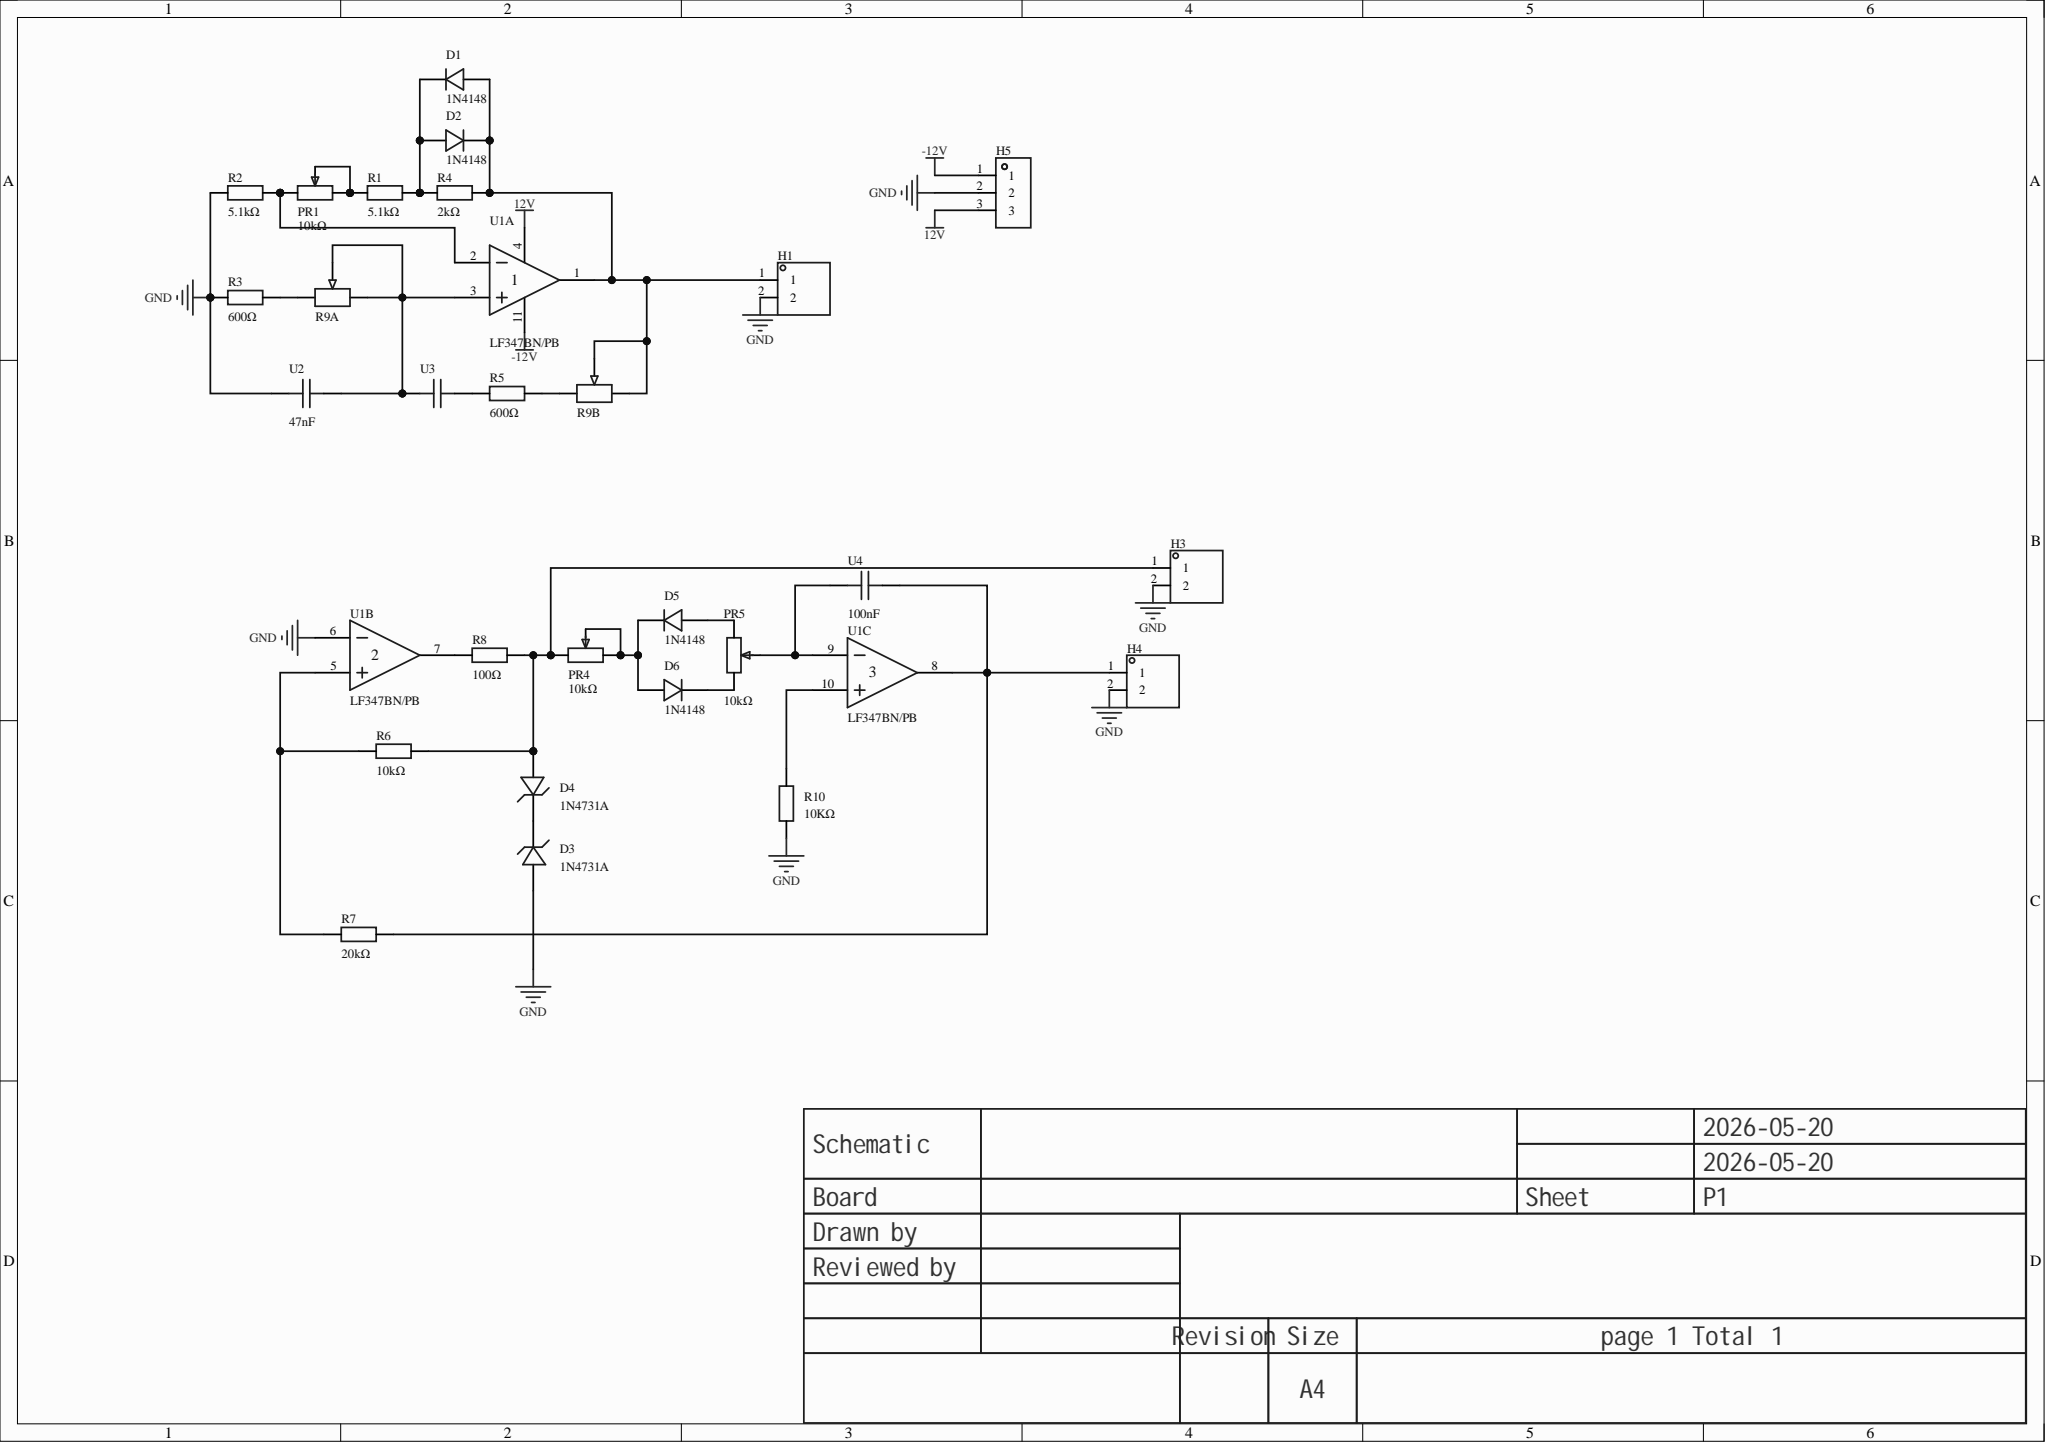Circuit board | Altium Designer | 27 parts | 21 nets
Bill of materials:
Comment,Description,Designator,Footprint,LibRef,Quantity
"1N4148","","D1, D2, D5, D6","DO-35_BD2.2-L4.0-D0.50_1N4148","1N4148_C9900036548","4"
"1N4731A","Diode configuration: standalone; Zener voltage (nominal): 4.3V; Zener voltage (range): 4.085V~4.515V; Power (Pd): 1W;","D3, D4","DO-41_BD2.4-L4.7-P8.70-D0.9-RD","1N4731A","2"
"","","H1, H3, H4","HDR-TH_2P-P2.54-V-M-1","HDR-M_2.54_1x2P","3"
"","","H5","HDR-TH_3P-P2.54-V-M","HDR-M_2.54_1x3P","1"
"10kΩ","","PR1, PR4, PR5","R_3296","R_3296","3"
"5.1kΩ","","R1, R2","Res_1/8W","Res_AXIAL-1/8W","2"
"600Ω","","R3, R5","Res_1/8W","Res_AXIAL-1/8W","2"
"2kΩ","","R4","Res_1/8W","Res_AXIAL-1/8W","1"
"10kΩ","","R6, R10","Res_1/8W","Res_AXIAL-1/8W","2"
"20kΩ","","R7","Res_1/8W","Res_AXIAL-1/8W","1"
"100Ω","","R8","Res_1/8W","Res_AXIAL-1/8W","1"
"","","R9","WH148","WH148","1"
"LF347BN/PB","Gain-bandwidth product (GBP): -; Input bias current (Ib): 50pA; Slew rate (SR): 13V/us;","U1","PDIP-14_L19.6-W6.5-P2.54-LS7.9-BL","LF347BN/PB","1"
"47nF","","U2, U3","CAP-TH_L5.0-W2.5-P5.00-D1.0","100nF","2"
"100nF","","U4","CAP-TH_L5.0-W2.5-P5.00-D1.0","100nF","1"
Netlist (Protel format):
[
D1
DO-35_BD2.2-L4.0-D0.50_1N4148
1N4148



]
[
D2
DO-35_BD2.2-L4.0-D0.50_1N4148
1N4148



]
[
D3
DO-41_BD2.4-L4.7-P8.70-D0.9-RD
1N4731A



]
[
D4
DO-41_BD2.4-L4.7-P8.70-D0.9-RD
1N4731A



]
[
D5
DO-35_BD2.2-L4.0-D0.50_1N4148
1N4148



]
[
D6
DO-35_BD2.2-L4.0-D0.50_1N4148
1N4148



]
[
H1
HDR-TH_2P-P2.54-V-M-1




]
[
H3
HDR-TH_2P-P2.54-V-M-1




]
[
H4
HDR-TH_2P-P2.54-V-M-1




]
[
H5
HDR-TH_3P-P2.54-V-M




]
[
PR1
R_3296
10kΩ



]
[
PR4
R_3296
10kΩ



]
[
PR5
R_3296
10kΩ



]
[
R1
Res_1/8W
5.1kΩ



]
[
R2
Res_1/8W
5.1kΩ



]
[
R3
Res_1/8W
600Ω



]
[
R4
Res_1/8W
2kΩ



]
[
R5
Res_1/8W
600Ω



]
[
R6
Res_1/8W
10kΩ



]
[
R7
Res_1/8W
20kΩ



]
[
R8
Res_1/8W
100Ω



]
[
R9
WH148




]
[
R10
Res_1/8W
10KΩ



]
[
U1
PDIP-14_L19.6-W6.5-P2.54-LS7.9-BL
LF347BN/PB



]
[
U2
CAP-TH_L5.0-W2.5-P5.00-D1.0
47nF



]
[
U3
CAP-TH_L5.0-W2.5-P5.00-D1.0
47nF



]
[
U4
CAP-TH_L5.0-W2.5-P5.00-D1.0
100nF



]
(
NetR10_2
R10-2
U1-10
)
(
NetR9_1
R9-1
R9-2
U1-3
U2-1
U3-2
)
(
NetR8_1
R8-1
U1-7
)
(
NetR6_1
R6-1
R7-1
U1-5
)
(
NetR5_2
R5-2
R9-4
)
(
NetR5_1
R5-1
U3-1
)
(
NetR3_2
R3-2
R9-3
)
(
NetPR5_2
PR5-2
U1-9
U4-2
)
(
NetPR1_3
PR1-3
R2-2
U1-2
)
(
NetPR1_1
PR1-1
PR1-2
R1-1
)
(
NetH4_1
H4-1
R7-2
U1-8
U4-1
)
(
NetD6_2
D6-2
PR5-1
)
(
NetD5_2
D5-2
D6-1
PR4-1
PR4-2
)
(
NetD5_1
D5-1
PR5-3
)
(
NetD4_2
D4-2
H3-1
PR4-3
R6-2
R8-2
)
(
NetD3_1
D3-1
D4-1
)
(
NetD1_2
D1-2
D2-1
R1-2
R4-1
)
(
NetD1_1
D1-1
D2-2
H1-1
R4-2
R9-5
R9-6
U1-1
)
(
GND
D3-2
H1-2
H3-2
H4-2
H5-2
R2-1
R3-1
R10-1
U1-6
U2-2
)
(
-12V
H5-1
U1-11
)
(
12V
H5-3
U1-4
)